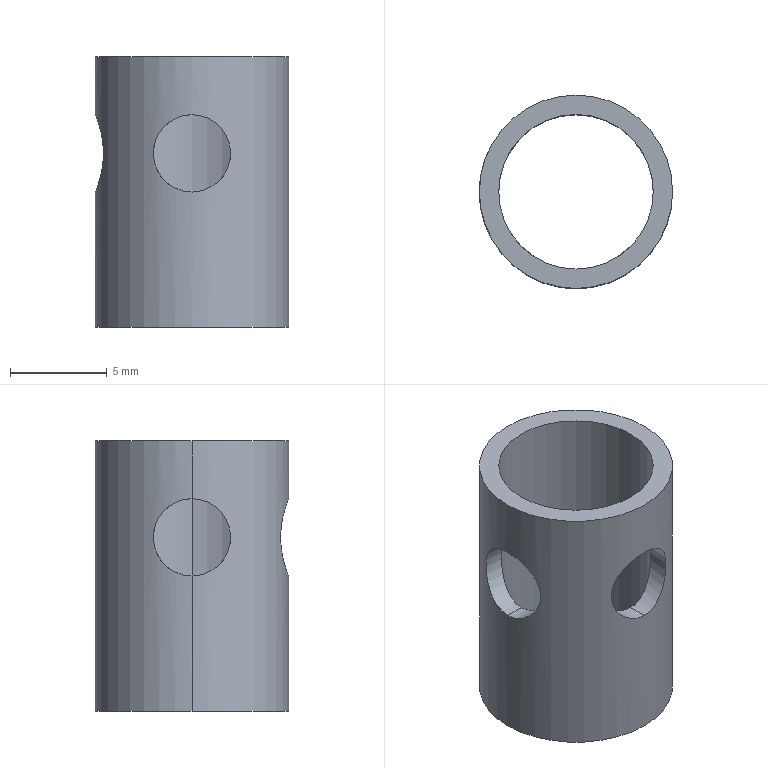Part | STEP file | 1 solid | 10 faces | box 10 x 10 x 14 mm | volume 370.028 mm3 | cylinder 8 | plane 2 | commonest cylinder face diameters 4 x4 8 x2 10 x2